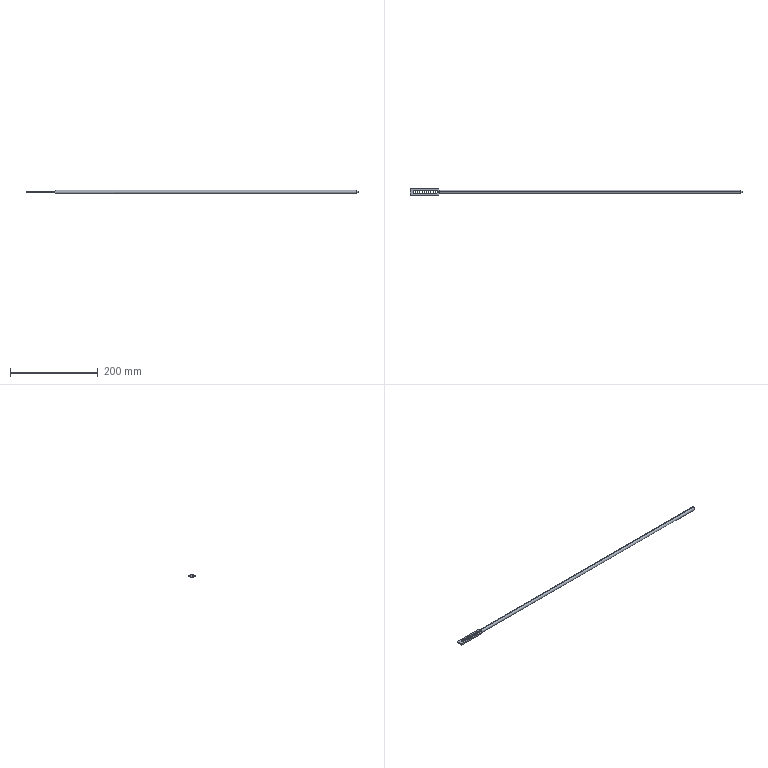Part | SolidWorks | 1 solid | 36 faces | box 757 x 14 x 8 mm | volume 36849 mm3 | cylinder 23 | plane 8 | cone 5 | commonest cylinder face diameters 6.1 x21 8 x2
STEP:
#1=CARTESIAN_POINT('',(67.,3.597,1.75));
#2=VERTEX_POINT('',#1);
#3=CARTESIAN_POINT('',(67.,0.,4.));
#4=VERTEX_POINT('',#3);
#5=CARTESIAN_POINT('',(67.,0.,0.));
#6=DIRECTION('',(1.,0.,0.));
#7=DIRECTION('',(0.,0.,-1.));
#8=AXIS2_PLACEMENT_3D('',#5,#6,#7);
#9=CIRCLE('',#8,4.);
#10=EDGE_CURVE('',#2,#4,#9,.T.);
#11=ORIENTED_EDGE('',*,*,#10,.T.);
#12=CARTESIAN_POINT('',(754.,0.,4.));
#13=VERTEX_POINT('',#12);
#14=CARTESIAN_POINT('',(757.,0.,4.));
#15=DIRECTION('',(1.,0.,0.));
#16=VECTOR('',#15,1000.);
#17=LINE('',#14,#16);
#18=EDGE_CURVE('',#4,#13,#17,.T.);
#19=ORIENTED_EDGE('',*,*,#18,.T.);
#20=CARTESIAN_POINT('',(754.,4.,0.));
#21=VERTEX_POINT('',#20);
#22=CARTESIAN_POINT('',(754.,0.,0.));
#23=DIRECTION('',(-1.,0.,0.));
#24=DIRECTION('',(0.,0.,-1.));
#25=AXIS2_PLACEMENT_3D('',#22,#23,#24);
#26=CIRCLE('',#25,4.);
#27=EDGE_CURVE('',#13,#21,#26,.T.);
#28=ORIENTED_EDGE('',*,*,#27,.T.);
#29=CARTESIAN_POINT('',(754.,0.,-4.));
#30=VERTEX_POINT('',#29);
#31=CARTESIAN_POINT('',(754.,0.,0.));
#32=DIRECTION('',(-1.,0.,0.));
#33=DIRECTION('',(0.,0.,-1.));
#34=AXIS2_PLACEMENT_3D('',#31,#32,#33);
#35=CIRCLE('',#34,4.);
#36=EDGE_CURVE('',#21,#30,#35,.T.);
#37=ORIENTED_EDGE('',*,*,#36,.T.);
#38=CARTESIAN_POINT('',(67.,0.,-4.));
#39=VERTEX_POINT('',#38);
#40=CARTESIAN_POINT('',(757.,0.,-4.));
#41=DIRECTION('',(1.,0.,0.));
#42=VECTOR('',#41,1000.);
#43=LINE('',#40,#42);
#44=EDGE_CURVE('',#39,#30,#43,.T.);
#45=ORIENTED_EDGE('',*,*,#44,.F.);
#46=CARTESIAN_POINT('',(67.,3.597,-1.75));
#47=VERTEX_POINT('',#46);
#48=CARTESIAN_POINT('',(67.,0.,0.));
#49=DIRECTION('',(1.,0.,0.));
#50=DIRECTION('',(0.,0.,-1.));
#51=AXIS2_PLACEMENT_3D('',#48,#49,#50);
#52=CIRCLE('',#51,4.);
#53=EDGE_CURVE('',#39,#47,#52,.T.);
#54=ORIENTED_EDGE('',*,*,#53,.T.);
#55=CARTESIAN_POINT('',(67.903,3.597,-1.75));
#56=VERTEX_POINT('',#55);
#57=CARTESIAN_POINT('',(68.,3.597,-1.75));
#58=DIRECTION('',(1.,0.,0.));
#59=VECTOR('',#58,1000.);
#60=LINE('',#57,#59);
#61=EDGE_CURVE('',#47,#56,#60,.T.);
#62=ORIENTED_EDGE('',*,*,#61,.T.);
#63=CARTESIAN_POINT('',(67.903,3.597,1.75));
#64=VERTEX_POINT('',#63);
#65=CARTESIAN_POINT('',(67.903,3.597,-1.75));
#66=CARTESIAN_POINT('',(67.356,4.144,-0.6253));
#67=CARTESIAN_POINT('',(67.356,4.144,0.6253));
#68=CARTESIAN_POINT('',(67.903,3.597,1.75));
#69=(BOUNDED_CURVE()B_SPLINE_CURVE(3,(#65,#66,#67,#68),.UNSPECIFIED.,.F.,.F.)B_SPLINE_CURVE_WITH_KNOTS((4,4),(2.689,3.594),.UNSPECIFIED.)CURVE()GEOMETRIC_REPRESENTATION_ITEM()RATIONAL_B_SPLINE_CURVE((1.,0.9328,0.9328,1.))REPRESENTATION_ITEM(''));
#70=EDGE_CURVE('',#56,#64,#69,.T.);
#71=ORIENTED_EDGE('',*,*,#70,.T.);
#72=CARTESIAN_POINT('',(0.,3.597,1.75));
#73=DIRECTION('',(-1.,0.,0.));
#74=VECTOR('',#73,1000.);
#75=LINE('',#72,#74);
#76=EDGE_CURVE('',#64,#2,#75,.T.);
#77=ORIENTED_EDGE('',*,*,#76,.T.);
#78=EDGE_LOOP('',(#11,#19,#28,#37,#45,#54,#62,#71,#77));
#79=FACE_OUTER_BOUND('',#78,.T.);
#80=CARTESIAN_POINT('',(757.,0.,0.));
#81=DIRECTION('',(1.,0.,0.));
#82=DIRECTION('',(0.,0.,-1.));
#83=AXIS2_PLACEMENT_3D('',#80,#81,#82);
#84=CYLINDRICAL_SURFACE('',#83,4.);
#85=ADVANCED_FACE('',(#79),#84,.T.);
#86=CARTESIAN_POINT('',(67.,-3.597,-1.75));
#87=VERTEX_POINT('',#86);
#88=CARTESIAN_POINT('',(65.678,0.,-1.75));
#89=VERTEX_POINT('',#88);
#90=CARTESIAN_POINT('',(67.,-3.597,-1.75));
#91=CARTESIAN_POINT('',(66.849,-3.312,-1.75));
#92=CARTESIAN_POINT('',(66.701,-3.025,-1.75));
#93=CARTESIAN_POINT('',(66.416,-2.448,-1.75));
#94=CARTESIAN_POINT('',(66.277,-2.157,-1.75));
#95=CARTESIAN_POINT('',(66.024,-1.564,-1.75));
#96=CARTESIAN_POINT('',(65.907,-1.262,-1.75));
#97=CARTESIAN_POINT('',(65.777,-0.7984,-1.75));
#98=CARTESIAN_POINT('',(65.741,-0.642,-1.75));
#99=CARTESIAN_POINT('',(65.692,-0.3236,-1.75));
#100=CARTESIAN_POINT('',(65.678,-0.1604,-1.75));
#101=CARTESIAN_POINT('',(65.678,0.,-1.75));
#102=B_SPLINE_CURVE_WITH_KNOTS('',3,(#90,#91,#92,#93,#94,#95,#96,#97,#98,#99,#100,#101),.UNSPECIFIED.,.F.,.F.,(4,2,2,2,2,4),(0.,0.0009664,0.001933,0.002899,0.003382,0.003866),.UNSPECIFIED.);
#103=EDGE_CURVE('',#87,#89,#102,.T.);
#104=ORIENTED_EDGE('',*,*,#103,.T.);
#105=CARTESIAN_POINT('',(67.,0.,-4.));
#106=DIRECTION('',(0.5065,0.,-0.8622));
#107=VECTOR('',#106,1000.);
#108=LINE('',#105,#107);
#109=EDGE_CURVE('',#89,#39,#108,.T.);
#110=ORIENTED_EDGE('',*,*,#109,.T.);
#111=CARTESIAN_POINT('',(67.,0.,0.));
#112=DIRECTION('',(1.,0.,0.));
#113=DIRECTION('',(0.,0.,-1.));
#114=AXIS2_PLACEMENT_3D('',#111,#112,#113);
#115=CIRCLE('',#114,4.);
#116=EDGE_CURVE('',#87,#39,#115,.T.);
#117=ORIENTED_EDGE('',*,*,#116,.F.);
#118=EDGE_LOOP('',(#104,#110,#117));
#119=FACE_OUTER_BOUND('',#118,.T.);
#120=CARTESIAN_POINT('',(67.,0.,0.));
#121=DIRECTION('',(1.,0.,0.));
#122=DIRECTION('',(0.,0.,-1.));
#123=AXIS2_PLACEMENT_3D('',#120,#121,#122);
#124=CONICAL_SURFACE('',#123,4.,1.04);
#125=ADVANCED_FACE('',(#119),#124,.T.);
#126=CARTESIAN_POINT('',(757.,-1.5,0.));
#127=VERTEX_POINT('',#126);
#128=CARTESIAN_POINT('',(757.,1.5,0.));
#129=VERTEX_POINT('',#128);
#130=CARTESIAN_POINT('',(757.,0.,0.));
#131=DIRECTION('',(-1.,0.,0.));
#132=DIRECTION('',(0.,-1.,0.));
#133=AXIS2_PLACEMENT_3D('',#130,#131,#132);
#134=CIRCLE('',#133,1.5);
#135=EDGE_CURVE('',#127,#129,#134,.T.);
#136=ORIENTED_EDGE('',*,*,#135,.T.);
#137=CARTESIAN_POINT('',(754.,4.,0.));
#138=DIRECTION('',(-0.7682,0.6402,0.));
#139=VECTOR('',#138,1000.);
#140=LINE('',#137,#139);
#141=EDGE_CURVE('',#129,#21,#140,.T.);
#142=ORIENTED_EDGE('',*,*,#141,.T.);
#143=ORIENTED_EDGE('',*,*,#27,.F.);
#144=CARTESIAN_POINT('',(754.,-4.,0.));
#145=VERTEX_POINT('',#144);
#146=CARTESIAN_POINT('',(754.,0.,0.));
#147=DIRECTION('',(-1.,0.,0.));
#148=DIRECTION('',(0.,0.,-1.));
#149=AXIS2_PLACEMENT_3D('',#146,#147,#148);
#150=CIRCLE('',#149,4.);
#151=EDGE_CURVE('',#145,#13,#150,.T.);
#152=ORIENTED_EDGE('',*,*,#151,.F.);
#153=CARTESIAN_POINT('',(754.,-4.,0.));
#154=DIRECTION('',(-0.7682,-0.6402,0.));
#155=VECTOR('',#154,1000.);
#156=LINE('',#153,#155);
#157=EDGE_CURVE('',#127,#145,#156,.T.);
#158=ORIENTED_EDGE('',*,*,#157,.F.);
#159=EDGE_LOOP('',(#136,#142,#143,#152,#158));
#160=FACE_OUTER_BOUND('',#159,.T.);
#161=CARTESIAN_POINT('',(754.,0.,0.));
#162=DIRECTION('',(-1.,0.,0.));
#163=DIRECTION('',(0.,-1.,0.));
#164=AXIS2_PLACEMENT_3D('',#161,#162,#163);
#165=CONICAL_SURFACE('',#164,4.,0.6947);
#166=ADVANCED_FACE('',(#160),#165,.T.);
#167=CARTESIAN_POINT('',(12.5,1.747,1.75));
#168=VERTEX_POINT('',#167);
#169=CARTESIAN_POINT('',(6.95,0.,1.75));
#170=VERTEX_POINT('',#169);
#171=CARTESIAN_POINT('',(10.,0.,1.75));
#172=DIRECTION('',(0.,0.,1.));
#173=DIRECTION('',(-1.,0.,0.));
#174=AXIS2_PLACEMENT_3D('',#171,#172,#173);
#175=CIRCLE('',#174,3.05);
#176=EDGE_CURVE('',#168,#170,#175,.T.);
#177=ORIENTED_EDGE('',*,*,#176,.T.);
#178=CARTESIAN_POINT('',(6.95,0.,-1.75));
#179=VERTEX_POINT('',#178);
#180=CARTESIAN_POINT('',(6.95,0.,7.));
#181=DIRECTION('',(0.,0.,-1.));
#182=VECTOR('',#181,1000.);
#183=LINE('',#180,#182);
#184=EDGE_CURVE('',#170,#179,#183,.T.);
#185=ORIENTED_EDGE('',*,*,#184,.T.);
#186=CARTESIAN_POINT('',(12.5,1.747,-1.75));
#187=VERTEX_POINT('',#186);
#188=CARTESIAN_POINT('',(10.,0.,-1.75));
#189=DIRECTION('',(0.,0.,-1.));
#190=DIRECTION('',(-1.,0.,0.));
#191=AXIS2_PLACEMENT_3D('',#188,#189,#190);
#192=CIRCLE('',#191,3.05);
#193=EDGE_CURVE('',#179,#187,#192,.T.);
#194=ORIENTED_EDGE('',*,*,#193,.T.);
#195=CARTESIAN_POINT('',(12.5,1.747,7.));
#196=DIRECTION('',(0.,0.,1.));
#197=VECTOR('',#196,1000.);
#198=LINE('',#195,#197);
#199=EDGE_CURVE('',#187,#168,#198,.T.);
#200=ORIENTED_EDGE('',*,*,#199,.T.);
#201=EDGE_LOOP('',(#177,#185,#194,#200));
#202=FACE_OUTER_BOUND('',#201,.T.);
#203=CARTESIAN_POINT('',(10.,0.,7.));
#204=DIRECTION('',(0.,0.,-1.));
#205=DIRECTION('',(-1.,0.,0.));
#206=AXIS2_PLACEMENT_3D('',#203,#204,#205);
#207=CYLINDRICAL_SURFACE('',#206,3.05);
#208=ADVANCED_FACE('',(#202),#207,.F.);
#209=ORIENTED_EDGE('',*,*,#18,.F.);
#210=CARTESIAN_POINT('',(67.,-3.597,1.75));
#211=VERTEX_POINT('',#210);
#212=CARTESIAN_POINT('',(67.,0.,0.));
#213=DIRECTION('',(1.,0.,0.));
#214=DIRECTION('',(0.,0.,-1.));
#215=AXIS2_PLACEMENT_3D('',#212,#213,#214);
#216=CIRCLE('',#215,4.);
#217=EDGE_CURVE('',#4,#211,#216,.T.);
#218=ORIENTED_EDGE('',*,*,#217,.T.);
#219=CARTESIAN_POINT('',(67.903,-3.597,1.75));
#220=VERTEX_POINT('',#219);
#221=CARTESIAN_POINT('',(0.,-3.597,1.75));
#222=DIRECTION('',(1.,0.,0.));
#223=VECTOR('',#222,1000.);
#224=LINE('',#221,#223);
#225=EDGE_CURVE('',#211,#220,#224,.T.);
#226=ORIENTED_EDGE('',*,*,#225,.T.);
#227=CARTESIAN_POINT('',(67.903,-3.597,-1.75));
#228=VERTEX_POINT('',#227);
#229=CARTESIAN_POINT('',(67.903,-3.597,1.75));
#230=CARTESIAN_POINT('',(67.356,-4.144,0.6253));
#231=CARTESIAN_POINT('',(67.356,-4.144,-0.6253));
#232=CARTESIAN_POINT('',(67.903,-3.597,-1.75));
#233=(BOUNDED_CURVE()B_SPLINE_CURVE(3,(#229,#230,#231,#232),.UNSPECIFIED.,.F.,.T.)B_SPLINE_CURVE_WITH_KNOTS((4,4),(2.689,3.594),.UNSPECIFIED.)CURVE()GEOMETRIC_REPRESENTATION_ITEM()RATIONAL_B_SPLINE_CURVE((1.,0.9328,0.9328,1.))REPRESENTATION_ITEM(''));
#234=EDGE_CURVE('',#220,#228,#233,.T.);
#235=ORIENTED_EDGE('',*,*,#234,.T.);
#236=CARTESIAN_POINT('',(68.,-3.597,-1.75));
#237=DIRECTION('',(-1.,0.,0.));
#238=VECTOR('',#237,1000.);
#239=LINE('',#236,#238);
#240=EDGE_CURVE('',#228,#87,#239,.T.);
#241=ORIENTED_EDGE('',*,*,#240,.T.);
#242=ORIENTED_EDGE('',*,*,#116,.T.);
#243=ORIENTED_EDGE('',*,*,#44,.T.);
#244=CARTESIAN_POINT('',(754.,0.,0.));
#245=DIRECTION('',(-1.,0.,0.));
#246=DIRECTION('',(0.,0.,-1.));
#247=AXIS2_PLACEMENT_3D('',#244,#245,#246);
#248=CIRCLE('',#247,4.);
#249=EDGE_CURVE('',#30,#145,#248,.T.);
#250=ORIENTED_EDGE('',*,*,#249,.T.);
#251=ORIENTED_EDGE('',*,*,#151,.T.);
#252=EDGE_LOOP('',(#209,#218,#226,#235,#241,#242,#243,#250,#251));
#253=FACE_OUTER_BOUND('',#252,.T.);
#254=CARTESIAN_POINT('',(757.,0.,0.));
#255=DIRECTION('',(1.,0.,0.));
#256=DIRECTION('',(0.,0.,-1.));
#257=AXIS2_PLACEMENT_3D('',#254,#255,#256);
#258=CYLINDRICAL_SURFACE('',#257,4.);
#259=ADVANCED_FACE('',(#253),#258,.T.);
#260=ORIENTED_EDGE('',*,*,#234,.F.);
#261=CARTESIAN_POINT('',(64.5,-7.,1.75));
#262=VERTEX_POINT('',#261);
#263=CARTESIAN_POINT('',(68.,-3.5,1.75));
#264=DIRECTION('',(0.7071,0.7071,0.));
#265=VECTOR('',#264,1000.);
#266=LINE('',#263,#265);
#267=EDGE_CURVE('',#262,#220,#266,.T.);
#268=ORIENTED_EDGE('',*,*,#267,.F.);
#269=CARTESIAN_POINT('',(64.5,-7.,-1.75));
#270=VERTEX_POINT('',#269);
#271=CARTESIAN_POINT('',(64.5,-7.,1.75));
#272=DIRECTION('',(0.,0.,1.));
#273=VECTOR('',#272,1000.);
#274=LINE('',#271,#273);
#275=EDGE_CURVE('',#270,#262,#274,.T.);
#276=ORIENTED_EDGE('',*,*,#275,.F.);
#277=CARTESIAN_POINT('',(68.,-3.5,-1.75));
#278=DIRECTION('',(-0.7071,-0.7071,0.));
#279=VECTOR('',#278,1000.);
#280=LINE('',#277,#279);
#281=EDGE_CURVE('',#228,#270,#280,.T.);
#282=ORIENTED_EDGE('',*,*,#281,.F.);
#283=EDGE_LOOP('',(#260,#268,#276,#282));
#284=FACE_OUTER_BOUND('',#283,.T.);
#285=CARTESIAN_POINT('',(68.,-3.5,1.75));
#286=DIRECTION('',(-0.7071,0.7071,0.));
#287=DIRECTION('',(-0.7071,-0.7071,0.));
#288=AXIS2_PLACEMENT_3D('',#285,#286,#287);
#289=PLANE('',#288);
#290=ADVANCED_FACE('',(#284),#289,.F.);
#291=ORIENTED_EDGE('',*,*,#10,.F.);
#292=CARTESIAN_POINT('',(67.,3.597,1.75));
#293=CARTESIAN_POINT('',(66.849,3.311,1.75));
#294=CARTESIAN_POINT('',(66.701,3.024,1.75));
#295=CARTESIAN_POINT('',(66.414,2.445,1.75));
#296=CARTESIAN_POINT('',(66.276,2.153,1.75));
#297=CARTESIAN_POINT('',(66.022,1.559,1.75));
#298=CARTESIAN_POINT('',(65.905,1.255,1.75));
#299=CARTESIAN_POINT('',(65.775,0.7905,1.75));
#300=CARTESIAN_POINT('',(65.74,0.6336,1.75));
#301=CARTESIAN_POINT('',(65.691,0.3142,1.75));
#302=CARTESIAN_POINT('',(65.678,0.1505,1.75));
#303=CARTESIAN_POINT('',(65.679,-0.3318,1.75));
#304=CARTESIAN_POINT('',(65.734,-0.6464,1.75));
#305=CARTESIAN_POINT('',(65.909,-1.267,1.75));
#306=CARTESIAN_POINT('',(66.026,-1.569,1.75));
#307=CARTESIAN_POINT('',(66.279,-2.16,1.75));
#308=CARTESIAN_POINT('',(66.417,-2.45,1.75));
#309=CARTESIAN_POINT('',(66.702,-3.027,1.75));
#310=CARTESIAN_POINT('',(66.85,-3.312,1.75));
#311=CARTESIAN_POINT('',(67.,-3.597,1.75));
#312=B_SPLINE_CURVE_WITH_KNOTS('',3,(#292,#293,#294,#295,#296,#297,#298,#299,#300,#301,#302,#303,#304,#305,#306,#307,#308,#309,#310,#311),.UNSPECIFIED.,.F.,.F.,(4,2,2,2,2,2,2,2,2,4),(0.,0.000969,0.001938,0.002907,0.003392,0.003876,0.004845,0.005814,0.006783,0.007752),.UNSPECIFIED.);
#313=EDGE_CURVE('',#2,#211,#312,.T.);
#314=ORIENTED_EDGE('',*,*,#313,.T.);
#315=ORIENTED_EDGE('',*,*,#217,.F.);
#316=EDGE_LOOP('',(#291,#314,#315));
#317=FACE_OUTER_BOUND('',#316,.T.);
#318=CARTESIAN_POINT('',(67.,0.,0.));
#319=DIRECTION('',(1.,0.,0.));
#320=DIRECTION('',(0.,0.,-1.));
#321=AXIS2_PLACEMENT_3D('',#318,#319,#320);
#322=CONICAL_SURFACE('',#321,4.,1.04);
#323=ADVANCED_FACE('',(#317),#322,.T.);
#324=CARTESIAN_POINT('',(64.5,7.,-1.75));
#325=VERTEX_POINT('',#324);
#326=CARTESIAN_POINT('',(64.5,7.,-1.75));
#327=DIRECTION('',(-0.7071,0.7071,0.));
#328=VECTOR('',#327,1000.);
#329=LINE('',#326,#328);
#330=EDGE_CURVE('',#56,#325,#329,.T.);
#331=ORIENTED_EDGE('',*,*,#330,.T.);
#332=CARTESIAN_POINT('',(64.5,7.,1.75));
#333=VERTEX_POINT('',#332);
#334=CARTESIAN_POINT('',(64.5,7.,0.));
#335=DIRECTION('',(0.,0.,1.));
#336=VECTOR('',#335,1000.);
#337=LINE('',#334,#336);
#338=EDGE_CURVE('',#325,#333,#337,.T.);
#339=ORIENTED_EDGE('',*,*,#338,.T.);
#340=CARTESIAN_POINT('',(64.5,7.,1.75));
#341=DIRECTION('',(0.7071,-0.7071,0.));
#342=VECTOR('',#341,1000.);
#343=LINE('',#340,#342);
#344=EDGE_CURVE('',#333,#64,#343,.T.);
#345=ORIENTED_EDGE('',*,*,#344,.T.);
#346=ORIENTED_EDGE('',*,*,#70,.F.);
#347=EDGE_LOOP('',(#331,#339,#345,#346));
#348=FACE_OUTER_BOUND('',#347,.T.);
#349=CARTESIAN_POINT('',(64.5,7.,0.));
#350=DIRECTION('',(0.7071,0.7071,0.));
#351=DIRECTION('',(-0.7071,0.7071,0.));
#352=AXIS2_PLACEMENT_3D('',#349,#350,#351);
#353=PLANE('',#352);
#354=ADVANCED_FACE('',(#348),#353,.T.);
#355=ORIENTED_EDGE('',*,*,#109,.F.);
#356=CARTESIAN_POINT('',(65.678,0.,-1.75));
#357=CARTESIAN_POINT('',(65.678,0.3225,-1.75));
#358=CARTESIAN_POINT('',(65.732,0.6381,-1.75));
#359=CARTESIAN_POINT('',(65.907,1.261,-1.75));
#360=CARTESIAN_POINT('',(66.024,1.564,-1.75));
#361=CARTESIAN_POINT('',(66.277,2.156,-1.75));
#362=CARTESIAN_POINT('',(66.415,2.447,-1.75));
#363=CARTESIAN_POINT('',(66.701,3.025,-1.75));
#364=CARTESIAN_POINT('',(66.849,3.312,-1.75));
#365=CARTESIAN_POINT('',(67.,3.597,-1.75));
#366=B_SPLINE_CURVE_WITH_KNOTS('',3,(#356,#357,#358,#359,#360,#361,#362,#363,#364,#365),.UNSPECIFIED.,.F.,.F.,(4,2,2,2,4),(0.003866,0.004837,0.005809,0.00678,0.007752),.UNSPECIFIED.);
#367=EDGE_CURVE('',#89,#47,#366,.T.);
#368=ORIENTED_EDGE('',*,*,#367,.T.);
#369=ORIENTED_EDGE('',*,*,#53,.F.);
#370=EDGE_LOOP('',(#355,#368,#369));
#371=FACE_OUTER_BOUND('',#370,.T.);
#372=CARTESIAN_POINT('',(67.,0.,0.));
#373=DIRECTION('',(1.,0.,0.));
#374=DIRECTION('',(0.,0.,-1.));
#375=AXIS2_PLACEMENT_3D('',#372,#373,#374);
#376=CONICAL_SURFACE('',#375,4.,1.04);
#377=ADVANCED_FACE('',(#371),#376,.T.);
#378=ORIENTED_EDGE('',*,*,#141,.F.);
#379=CARTESIAN_POINT('',(757.,0.,0.));
#380=DIRECTION('',(-1.,0.,0.));
#381=DIRECTION('',(0.,-1.,0.));
#382=AXIS2_PLACEMENT_3D('',#379,#380,#381);
#383=CIRCLE('',#382,1.5);
#384=EDGE_CURVE('',#129,#127,#383,.T.);
#385=ORIENTED_EDGE('',*,*,#384,.T.);
#386=ORIENTED_EDGE('',*,*,#157,.T.);
#387=ORIENTED_EDGE('',*,*,#249,.F.);
#388=ORIENTED_EDGE('',*,*,#36,.F.);
#389=EDGE_LOOP('',(#378,#385,#386,#387,#388));
#390=FACE_OUTER_BOUND('',#389,.T.);
#391=CARTESIAN_POINT('',(754.,0.,0.));
#392=DIRECTION('',(-1.,0.,0.));
#393=DIRECTION('',(0.,-1.,0.));
#394=AXIS2_PLACEMENT_3D('',#391,#392,#393);
#395=CONICAL_SURFACE('',#394,4.,0.6947);
#396=ADVANCED_FACE('',(#390),#395,.T.);
#397=ORIENTED_EDGE('',*,*,#281,.T.);
#398=CARTESIAN_POINT('',(0.,-7.,-1.75));
#399=VERTEX_POINT('',#398);
#400=CARTESIAN_POINT('',(68.,-7.,-1.75));
#401=DIRECTION('',(1.,0.,0.));
#402=VECTOR('',#401,1000.);
#403=LINE('',#400,#402);
#404=EDGE_CURVE('',#399,#270,#403,.T.);
#405=ORIENTED_EDGE('',*,*,#404,.F.);
#406=CARTESIAN_POINT('',(0.,7.,-1.75));
#407=VERTEX_POINT('',#406);
#408=CARTESIAN_POINT('',(0.,7.,-1.75));
#409=DIRECTION('',(0.,-1.,0.));
#410=VECTOR('',#409,1000.);
#411=LINE('',#408,#410);
#412=EDGE_CURVE('',#407,#399,#411,.T.);
#413=ORIENTED_EDGE('',*,*,#412,.F.);
#414=CARTESIAN_POINT('',(68.,7.,-1.75));
#415=DIRECTION('',(-1.,0.,0.));
#416=VECTOR('',#415,1000.);
#417=LINE('',#414,#416);
#418=EDGE_CURVE('',#325,#407,#417,.T.);
#419=ORIENTED_EDGE('',*,*,#418,.F.);
#420=ORIENTED_EDGE('',*,*,#330,.F.);
#421=ORIENTED_EDGE('',*,*,#61,.F.);
#422=ORIENTED_EDGE('',*,*,#367,.F.);
#423=ORIENTED_EDGE('',*,*,#103,.F.);
#424=ORIENTED_EDGE('',*,*,#240,.F.);
#425=EDGE_LOOP('',(#397,#405,#413,#419,#420,#421,#422,#423,#424));
#426=FACE_OUTER_BOUND('',#425,.T.);
#427=CARTESIAN_POINT('',(22.5,-1.747,-1.75));
#428=VERTEX_POINT('',#427);
#429=CARTESIAN_POINT('',(17.5,-1.747,-1.75));
#430=VERTEX_POINT('',#429);
#431=CARTESIAN_POINT('',(20.,0.,-1.75));
#432=DIRECTION('',(0.,0.,-1.));
#433=DIRECTION('',(-1.,0.,0.));
#434=AXIS2_PLACEMENT_3D('',#431,#432,#433);
#435=CIRCLE('',#434,3.05);
#436=EDGE_CURVE('',#428,#430,#435,.T.);
#437=ORIENTED_EDGE('',*,*,#436,.F.);
#438=CARTESIAN_POINT('',(27.5,-1.747,-1.75));
#439=VERTEX_POINT('',#438);
#440=CARTESIAN_POINT('',(25.,0.,-1.75));
#441=DIRECTION('',(0.,0.,-1.));
#442=DIRECTION('',(-1.,0.,0.));
#443=AXIS2_PLACEMENT_3D('',#440,#441,#442);
#444=CIRCLE('',#443,3.05);
#445=EDGE_CURVE('',#439,#428,#444,.T.);
#446=ORIENTED_EDGE('',*,*,#445,.F.);
#447=CARTESIAN_POINT('',(32.5,-1.747,-1.75));
#448=VERTEX_POINT('',#447);
#449=CARTESIAN_POINT('',(30.,0.,-1.75));
#450=DIRECTION('',(0.,0.,-1.));
#451=DIRECTION('',(-1.,0.,0.));
#452=AXIS2_PLACEMENT_3D('',#449,#450,#451);
#453=CIRCLE('',#452,3.05);
#454=EDGE_CURVE('',#448,#439,#453,.T.);
#455=ORIENTED_EDGE('',*,*,#454,.F.);
#456=CARTESIAN_POINT('',(37.5,-1.747,-1.75));
#457=VERTEX_POINT('',#456);
#458=CARTESIAN_POINT('',(35.,0.,-1.75));
#459=DIRECTION('',(0.,0.,-1.));
#460=DIRECTION('',(-1.,0.,0.));
#461=AXIS2_PLACEMENT_3D('',#458,#459,#460);
#462=CIRCLE('',#461,3.05);
#463=EDGE_CURVE('',#457,#448,#462,.T.);
#464=ORIENTED_EDGE('',*,*,#463,.F.);
#465=CARTESIAN_POINT('',(42.5,-1.747,-1.75));
#466=VERTEX_POINT('',#465);
#467=CARTESIAN_POINT('',(40.,0.,-1.75));
#468=DIRECTION('',(0.,0.,-1.));
#469=DIRECTION('',(-1.,0.,0.));
#470=AXIS2_PLACEMENT_3D('',#467,#468,#469);
#471=CIRCLE('',#470,3.05);
#472=EDGE_CURVE('',#466,#457,#471,.T.);
#473=ORIENTED_EDGE('',*,*,#472,.F.);
#474=CARTESIAN_POINT('',(47.5,-1.747,-1.75));
#475=VERTEX_POINT('',#474);
#476=CARTESIAN_POINT('',(45.,0.,-1.75));
#477=DIRECTION('',(0.,0.,-1.));
#478=DIRECTION('',(-1.,0.,0.));
#479=AXIS2_PLACEMENT_3D('',#476,#477,#478);
#480=CIRCLE('',#479,3.05);
#481=EDGE_CURVE('',#475,#466,#480,.T.);
#482=ORIENTED_EDGE('',*,*,#481,.F.);
#483=CARTESIAN_POINT('',(52.5,-1.747,-1.75));
#484=VERTEX_POINT('',#483);
#485=CARTESIAN_POINT('',(50.,0.,-1.75));
#486=DIRECTION('',(0.,0.,-1.));
#487=DIRECTION('',(-1.,0.,0.));
#488=AXIS2_PLACEMENT_3D('',#485,#486,#487);
#489=CIRCLE('',#488,3.05);
#490=EDGE_CURVE('',#484,#475,#489,.T.);
#491=ORIENTED_EDGE('',*,*,#490,.F.);
#492=CARTESIAN_POINT('',(57.5,-1.747,-1.75));
#493=VERTEX_POINT('',#492);
#494=CARTESIAN_POINT('',(55.,0.,-1.75));
#495=DIRECTION('',(0.,0.,-1.));
#496=DIRECTION('',(-1.,0.,0.));
#497=AXIS2_PLACEMENT_3D('',#494,#495,#496);
#498=CIRCLE('',#497,3.05);
#499=EDGE_CURVE('',#493,#484,#498,.T.);
#500=ORIENTED_EDGE('',*,*,#499,.F.);
#501=CARTESIAN_POINT('',(57.5,1.747,-1.75));
#502=VERTEX_POINT('',#501);
#503=CARTESIAN_POINT('',(60.,0.,-1.75));
#504=DIRECTION('',(0.,0.,-1.));
#505=DIRECTION('',(-1.,0.,0.));
#506=AXIS2_PLACEMENT_3D('',#503,#504,#505);
#507=CIRCLE('',#506,3.05);
#508=EDGE_CURVE('',#502,#493,#507,.T.);
#509=ORIENTED_EDGE('',*,*,#508,.F.);
#510=CARTESIAN_POINT('',(52.5,1.747,-1.75));
#511=VERTEX_POINT('',#510);
#512=CARTESIAN_POINT('',(55.,0.,-1.75));
#513=DIRECTION('',(0.,0.,-1.));
#514=DIRECTION('',(-1.,0.,0.));
#515=AXIS2_PLACEMENT_3D('',#512,#513,#514);
#516=CIRCLE('',#515,3.05);
#517=EDGE_CURVE('',#511,#502,#516,.T.);
#518=ORIENTED_EDGE('',*,*,#517,.F.);
#519=CARTESIAN_POINT('',(47.5,1.747,-1.75));
#520=VERTEX_POINT('',#519);
#521=CARTESIAN_POINT('',(50.,0.,-1.75));
#522=DIRECTION('',(0.,0.,-1.));
#523=DIRECTION('',(-1.,0.,0.));
#524=AXIS2_PLACEMENT_3D('',#521,#522,#523);
#525=CIRCLE('',#524,3.05);
#526=EDGE_CURVE('',#520,#511,#525,.T.);
#527=ORIENTED_EDGE('',*,*,#526,.F.);
#528=CARTESIAN_POINT('',(42.5,1.747,-1.75));
#529=VERTEX_POINT('',#528);
#530=CARTESIAN_POINT('',(45.,0.,-1.75));
#531=DIRECTION('',(0.,0.,-1.));
#532=DIRECTION('',(-1.,0.,0.));
#533=AXIS2_PLACEMENT_3D('',#530,#531,#532);
#534=CIRCLE('',#533,3.05);
#535=EDGE_CURVE('',#529,#520,#534,.T.);
#536=ORIENTED_EDGE('',*,*,#535,.F.);
#537=CARTESIAN_POINT('',(37.5,1.747,-1.75));
#538=VERTEX_POINT('',#537);
#539=CARTESIAN_POINT('',(40.,0.,-1.75));
#540=DIRECTION('',(0.,0.,-1.));
#541=DIRECTION('',(-1.,0.,0.));
#542=AXIS2_PLACEMENT_3D('',#539,#540,#541);
#543=CIRCLE('',#542,3.05);
#544=EDGE_CURVE('',#538,#529,#543,.T.);
#545=ORIENTED_EDGE('',*,*,#544,.F.);
#546=CARTESIAN_POINT('',(32.5,1.747,-1.75));
#547=VERTEX_POINT('',#546);
#548=CARTESIAN_POINT('',(35.,0.,-1.75));
#549=DIRECTION('',(0.,0.,-1.));
#550=DIRECTION('',(-1.,0.,0.));
#551=AXIS2_PLACEMENT_3D('',#548,#549,#550);
#552=CIRCLE('',#551,3.05);
#553=EDGE_CURVE('',#547,#538,#552,.T.);
#554=ORIENTED_EDGE('',*,*,#553,.F.);
#555=CARTESIAN_POINT('',(27.5,1.747,-1.75));
#556=VERTEX_POINT('',#555);
#557=CARTESIAN_POINT('',(30.,0.,-1.75));
#558=DIRECTION('',(0.,0.,-1.));
#559=DIRECTION('',(-1.,0.,0.));
#560=AXIS2_PLACEMENT_3D('',#557,#558,#559);
#561=CIRCLE('',#560,3.05);
#562=EDGE_CURVE('',#556,#547,#561,.T.);
#563=ORIENTED_EDGE('',*,*,#562,.F.);
#564=CARTESIAN_POINT('',(22.5,1.747,-1.75));
#565=VERTEX_POINT('',#564);
#566=CARTESIAN_POINT('',(25.,0.,-1.75));
#567=DIRECTION('',(0.,0.,-1.));
#568=DIRECTION('',(-1.,0.,0.));
#569=AXIS2_PLACEMENT_3D('',#566,#567,#568);
#570=CIRCLE('',#569,3.05);
#571=EDGE_CURVE('',#565,#556,#570,.T.);
#572=ORIENTED_EDGE('',*,*,#571,.F.);
#573=CARTESIAN_POINT('',(17.5,1.747,-1.75));
#574=VERTEX_POINT('',#573);
#575=CARTESIAN_POINT('',(20.,0.,-1.75));
#576=DIRECTION('',(0.,0.,-1.));
#577=DIRECTION('',(-1.,0.,0.));
#578=AXIS2_PLACEMENT_3D('',#575,#576,#577);
#579=CIRCLE('',#578,3.05);
#580=EDGE_CURVE('',#574,#565,#579,.T.);
#581=ORIENTED_EDGE('',*,*,#580,.F.);
#582=CARTESIAN_POINT('',(15.,0.,-1.75));
#583=DIRECTION('',(0.,0.,-1.));
#584=DIRECTION('',(-1.,0.,0.));
#585=AXIS2_PLACEMENT_3D('',#582,#583,#584);
#586=CIRCLE('',#585,3.05);
#587=EDGE_CURVE('',#187,#574,#586,.T.);
#588=ORIENTED_EDGE('',*,*,#587,.F.);
#589=ORIENTED_EDGE('',*,*,#193,.F.);
#590=CARTESIAN_POINT('',(12.5,-1.747,-1.75));
#591=VERTEX_POINT('',#590);
#592=CARTESIAN_POINT('',(10.,0.,-1.75));
#593=DIRECTION('',(0.,0.,-1.));
#594=DIRECTION('',(-1.,0.,0.));
#595=AXIS2_PLACEMENT_3D('',#592,#593,#594);
#596=CIRCLE('',#595,3.05);
#597=EDGE_CURVE('',#591,#179,#596,.T.);
#598=ORIENTED_EDGE('',*,*,#597,.F.);
#599=CARTESIAN_POINT('',(15.,0.,-1.75));
#600=DIRECTION('',(0.,0.,-1.));
#601=DIRECTION('',(-1.,0.,0.));
#602=AXIS2_PLACEMENT_3D('',#599,#600,#601);
#603=CIRCLE('',#602,3.05);
#604=EDGE_CURVE('',#430,#591,#603,.T.);
#605=ORIENTED_EDGE('',*,*,#604,.F.);
#606=EDGE_LOOP('',(#437,#446,#455,#464,#473,#482,#491,#500,#509,#518,#527,#536,#545,#554,#563,#572,#581,#588,#589,#598,#605));
#607=FACE_BOUND('',#606,.T.);
#608=CARTESIAN_POINT('',(68.,7.,-1.75));
#609=DIRECTION('',(0.,0.,1.));
#610=DIRECTION('',(1.,0.,0.));
#611=AXIS2_PLACEMENT_3D('',#608,#609,#610);
#612=PLANE('',#611);
#613=ADVANCED_FACE('',(#426,#607),#612,.F.);
#614=ORIENTED_EDGE('',*,*,#344,.F.);
#615=CARTESIAN_POINT('',(0.,7.,1.75));
#616=VERTEX_POINT('',#615);
#617=CARTESIAN_POINT('',(0.,7.,1.75));
#618=DIRECTION('',(1.,0.,0.));
#619=VECTOR('',#618,1000.);
#620=LINE('',#617,#619);
#621=EDGE_CURVE('',#616,#333,#620,.T.);
#622=ORIENTED_EDGE('',*,*,#621,.F.);
#623=CARTESIAN_POINT('',(0.,-7.,1.75));
#624=VERTEX_POINT('',#623);
#625=CARTESIAN_POINT('',(0.,7.,1.75));
#626=DIRECTION('',(0.,1.,0.));
#627=VECTOR('',#626,1000.);
#628=LINE('',#625,#627);
#629=EDGE_CURVE('',#624,#616,#628,.T.);
#630=ORIENTED_EDGE('',*,*,#629,.F.);
#631=CARTESIAN_POINT('',(0.,-7.,1.75));
#632=DIRECTION('',(-1.,0.,0.));
#633=VECTOR('',#632,1000.);
#634=LINE('',#631,#633);
#635=EDGE_CURVE('',#262,#624,#634,.T.);
#636=ORIENTED_EDGE('',*,*,#635,.F.);
#637=ORIENTED_EDGE('',*,*,#267,.T.);
#638=ORIENTED_EDGE('',*,*,#225,.F.);
#639=ORIENTED_EDGE('',*,*,#313,.F.);
#640=ORIENTED_EDGE('',*,*,#76,.F.);
#641=EDGE_LOOP('',(#614,#622,#630,#636,#637,#638,#639,#640));
#642=FACE_OUTER_BOUND('',#641,.T.);
#643=CARTESIAN_POINT('',(22.5,1.747,1.75));
#644=VERTEX_POINT('',#643);
#645=CARTESIAN_POINT('',(17.5,1.747,1.75));
#646=VERTEX_POINT('',#645);
#647=CARTESIAN_POINT('',(20.,0.,1.75));
#648=DIRECTION('',(0.,0.,1.));
#649=DIRECTION('',(-1.,0.,0.));
#650=AXIS2_PLACEMENT_3D('',#647,#648,#649);
#651=CIRCLE('',#650,3.05);
#652=EDGE_CURVE('',#644,#646,#651,.T.);
#653=ORIENTED_EDGE('',*,*,#652,.F.);
#654=CARTESIAN_POINT('',(27.5,1.747,1.75));
#655=VERTEX_POINT('',#654);
#656=CARTESIAN_POINT('',(25.,0.,1.75));
#657=DIRECTION('',(0.,0.,1.));
#658=DIRECTION('',(-1.,0.,0.));
#659=AXIS2_PLACEMENT_3D('',#656,#657,#658);
#660=CIRCLE('',#659,3.05);
#661=EDGE_CURVE('',#655,#644,#660,.T.);
#662=ORIENTED_EDGE('',*,*,#661,.F.);
#663=CARTESIAN_POINT('',(32.5,1.747,1.75));
#664=VERTEX_POINT('',#663);
#665=CARTESIAN_POINT('',(30.,0.,1.75));
#666=DIRECTION('',(0.,0.,1.));
#667=DIRECTION('',(-1.,0.,0.));
#668=AXIS2_PLACEMENT_3D('',#665,#666,#667);
#669=CIRCLE('',#668,3.05);
#670=EDGE_CURVE('',#664,#655,#669,.T.);
#671=ORIENTED_EDGE('',*,*,#670,.F.);
#672=CARTESIAN_POINT('',(37.5,1.747,1.75));
#673=VERTEX_POINT('',#672);
#674=CARTESIAN_POINT('',(35.,0.,1.75));
#675=DIRECTION('',(0.,0.,1.));
#676=DIRECTION('',(-1.,0.,0.));
#677=AXIS2_PLACEMENT_3D('',#674,#675,#676);
#678=CIRCLE('',#677,3.05);
#679=EDGE_CURVE('',#673,#664,#678,.T.);
#680=ORIENTED_EDGE('',*,*,#679,.F.);
#681=CARTESIAN_POINT('',(42.5,1.747,1.75));
#682=VERTEX_POINT('',#681);
#683=CARTESIAN_POINT('',(40.,0.,1.75));
#684=DIRECTION('',(0.,0.,1.));
#685=DIRECTION('',(-1.,0.,0.));
#686=AXIS2_PLACEMENT_3D('',#683,#684,#685);
#687=CIRCLE('',#686,3.05);
#688=EDGE_CURVE('',#682,#673,#687,.T.);
#689=ORIENTED_EDGE('',*,*,#688,.F.);
#690=CARTESIAN_POINT('',(47.5,1.747,1.75));
#691=VERTEX_POINT('',#690);
#692=CARTESIAN_POINT('',(45.,0.,1.75));
#693=DIRECTION('',(0.,0.,1.));
#694=DIRECTION('',(-1.,0.,0.));
#695=AXIS2_PLACEMENT_3D('',#692,#693,#694);
#696=CIRCLE('',#695,3.05);
#697=EDGE_CURVE('',#691,#682,#696,.T.);
#698=ORIENTED_EDGE('',*,*,#697,.F.);
#699=CARTESIAN_POINT('',(52.5,1.747,1.75));
#700=VERTEX_POINT('',#699);
#701=CARTESIAN_POINT('',(50.,0.,1.75));
#702=DIRECTION('',(0.,0.,1.));
#703=DIRECTION('',(-1.,0.,0.));
#704=AXIS2_PLACEMENT_3D('',#701,#702,#703);
#705=CIRCLE('',#704,3.05);
#706=EDGE_CURVE('',#700,#691,#705,.T.);
#707=ORIENTED_EDGE('',*,*,#706,.F.);
#708=CARTESIAN_POINT('',(57.5,1.747,1.75));
#709=VERTEX_POINT('',#708);
#710=CARTESIAN_POINT('',(55.,0.,1.75));
#711=DIRECTION('',(0.,0.,1.));
#712=DIRECTION('',(-1.,0.,0.));
#713=AXIS2_PLACEMENT_3D('',#710,#711,#712);
#714=CIRCLE('',#713,3.05);
#715=EDGE_CURVE('',#709,#700,#714,.T.);
#716=ORIENTED_EDGE('',*,*,#715,.F.);
#717=CARTESIAN_POINT('',(57.5,-1.747,1.75));
#718=VERTEX_POINT('',#717);
#719=CARTESIAN_POINT('',(60.,0.,1.75));
#720=DIRECTION('',(0.,0.,1.));
#721=DIRECTION('',(-1.,0.,0.));
#722=AXIS2_PLACEMENT_3D('',#719,#720,#721);
#723=CIRCLE('',#722,3.05);
#724=EDGE_CURVE('',#718,#709,#723,.T.);
#725=ORIENTED_EDGE('',*,*,#724,.F.);
#726=CARTESIAN_POINT('',(52.5,-1.747,1.75));
#727=VERTEX_POINT('',#726);
#728=CARTESIAN_POINT('',(55.,0.,1.75));
#729=DIRECTION('',(0.,0.,1.));
#730=DIRECTION('',(-1.,0.,0.));
#731=AXIS2_PLACEMENT_3D('',#728,#729,#730);
#732=CIRCLE('',#731,3.05);
#733=EDGE_CURVE('',#727,#718,#732,.T.);
#734=ORIENTED_EDGE('',*,*,#733,.F.);
#735=CARTESIAN_POINT('',(47.5,-1.747,1.75));
#736=VERTEX_POINT('',#735);
#737=CARTESIAN_POINT('',(50.,0.,1.75));
#738=DIRECTION('',(0.,0.,1.));
#739=DIRECTION('',(-1.,0.,0.));
#740=AXIS2_PLACEMENT_3D('',#737,#738,#739);
#741=CIRCLE('',#740,3.05);
#742=EDGE_CURVE('',#736,#727,#741,.T.);
#743=ORIENTED_EDGE('',*,*,#742,.F.);
#744=CARTESIAN_POINT('',(42.5,-1.747,1.75));
#745=VERTEX_POINT('',#744);
#746=CARTESIAN_POINT('',(45.,0.,1.75));
#747=DIRECTION('',(0.,0.,1.));
#748=DIRECTION('',(-1.,0.,0.));
#749=AXIS2_PLACEMENT_3D('',#746,#747,#748);
#750=CIRCLE('',#749,3.05);
#751=EDGE_CURVE('',#745,#736,#750,.T.);
#752=ORIENTED_EDGE('',*,*,#751,.F.);
#753=CARTESIAN_POINT('',(37.5,-1.747,1.75));
#754=VERTEX_POINT('',#753);
#755=CARTESIAN_POINT('',(40.,0.,1.75));
#756=DIRECTION('',(0.,0.,1.));
#757=DIRECTION('',(-1.,0.,0.));
#758=AXIS2_PLACEMENT_3D('',#755,#756,#757);
#759=CIRCLE('',#758,3.05);
#760=EDGE_CURVE('',#754,#745,#759,.T.);
#761=ORIENTED_EDGE('',*,*,#760,.F.);
#762=CARTESIAN_POINT('',(32.5,-1.747,1.75));
#763=VERTEX_POINT('',#762);
#764=CARTESIAN_POINT('',(35.,0.,1.75));
#765=DIRECTION('',(0.,0.,1.));
#766=DIRECTION('',(-1.,0.,0.));
#767=AXIS2_PLACEMENT_3D('',#764,#765,#766);
#768=CIRCLE('',#767,3.05);
#769=EDGE_CURVE('',#763,#754,#768,.T.);
#770=ORIENTED_EDGE('',*,*,#769,.F.);
#771=CARTESIAN_POINT('',(27.5,-1.747,1.75));
#772=VERTEX_POINT('',#771);
#773=CARTESIAN_POINT('',(30.,0.,1.75));
#774=DIRECTION('',(0.,0.,1.));
#775=DIRECTION('',(-1.,0.,0.));
#776=AXIS2_PLACEMENT_3D('',#773,#774,#775);
#777=CIRCLE('',#776,3.05);
#778=EDGE_CURVE('',#772,#763,#777,.T.);
#779=ORIENTED_EDGE('',*,*,#778,.F.);
#780=CARTESIAN_POINT('',(22.5,-1.747,1.75));
#781=VERTEX_POINT('',#780);
#782=CARTESIAN_POINT('',(25.,0.,1.75));
#783=DIRECTION('',(0.,0.,1.));
#784=DIRECTION('',(-1.,0.,0.));
#785=AXIS2_PLACEMENT_3D('',#782,#783,#784);
#786=CIRCLE('',#785,3.05);
#787=EDGE_CURVE('',#781,#772,#786,.T.);
#788=ORIENTED_EDGE('',*,*,#787,.F.);
#789=CARTESIAN_POINT('',(17.5,-1.747,1.75));
#790=VERTEX_POINT('',#789);
#791=CARTESIAN_POINT('',(20.,0.,1.75));
#792=DIRECTION('',(0.,0.,1.));
#793=DIRECTION('',(-1.,0.,0.));
#794=AXIS2_PLACEMENT_3D('',#791,#792,#793);
#795=CIRCLE('',#794,3.05);
#796=EDGE_CURVE('',#790,#781,#795,.T.);
#797=ORIENTED_EDGE('',*,*,#796,.F.);
#798=CARTESIAN_POINT('',(12.5,-1.747,1.75));
#799=VERTEX_POINT('',#798);
#800=CARTESIAN_POINT('',(15.,0.,1.75));
#801=DIRECTION('',(0.,0.,1.));
#802=DIRECTION('',(-1.,0.,0.));
#803=AXIS2_PLACEMENT_3D('',#800,#801,#802);
#804=CIRCLE('',#803,3.05);
#805=EDGE_CURVE('',#799,#790,#804,.T.);
#806=ORIENTED_EDGE('',*,*,#805,.F.);
#807=CARTESIAN_POINT('',(10.,0.,1.75));
#808=DIRECTION('',(0.,0.,1.));
#809=DIRECTION('',(-1.,0.,0.));
#810=AXIS2_PLACEMENT_3D('',#807,#808,#809);
#811=CIRCLE('',#810,3.05);
#812=EDGE_CURVE('',#170,#799,#811,.T.);
#813=ORIENTED_EDGE('',*,*,#812,.F.);
#814=ORIENTED_EDGE('',*,*,#176,.F.);
#815=CARTESIAN_POINT('',(15.,0.,1.75));
#816=DIRECTION('',(0.,0.,1.));
#817=DIRECTION('',(-1.,0.,0.));
#818=AXIS2_PLACEMENT_3D('',#815,#816,#817);
#819=CIRCLE('',#818,3.05);
#820=EDGE_CURVE('',#646,#168,#819,.T.);
#821=ORIENTED_EDGE('',*,*,#820,.F.);
#822=EDGE_LOOP('',(#653,#662,#671,#680,#689,#698,#707,#716,#725,#734,#743,#752,#761,#770,#779,#788,#797,#806,#813,#814,#821));
#823=FACE_BOUND('',#822,.T.);
#824=CARTESIAN_POINT('',(0.,7.,1.75));
#825=DIRECTION('',(0.,0.,-1.));
#826=DIRECTION('',(-1.,0.,0.));
#827=AXIS2_PLACEMENT_3D('',#824,#825,#826);
#828=PLANE('',#827);
#829=ADVANCED_FACE('',(#642,#823),#828,.F.);
#830=ORIENTED_EDGE('',*,*,#275,.T.);
#831=ORIENTED_EDGE('',*,*,#635,.T.);
#832=CARTESIAN_POINT('',(0.,-7.,0.));
#833=DIRECTION('',(0.,0.,1.));
#834=VECTOR('',#833,1000.);
#835=LINE('',#832,#834);
#836=EDGE_CURVE('',#399,#624,#835,.T.);
#837=ORIENTED_EDGE('',*,*,#836,.F.);
#838=ORIENTED_EDGE('',*,*,#404,.T.);
#839=EDGE_LOOP('',(#830,#831,#837,#838));
#840=FACE_OUTER_BOUND('',#839,.T.);
#841=CARTESIAN_POINT('',(0.,-7.,0.));
#842=DIRECTION('',(0.,1.,0.));
#843=DIRECTION('',(0.,0.,1.));
#844=AXIS2_PLACEMENT_3D('',#841,#842,#843);
#845=PLANE('',#844);
#846=ADVANCED_FACE('',(#840),#845,.F.);
#847=ORIENTED_EDGE('',*,*,#418,.T.);
#848=CARTESIAN_POINT('',(0.,7.,0.));
#849=DIRECTION('',(0.,0.,1.));
#850=VECTOR('',#849,1000.);
#851=LINE('',#848,#850);
#852=EDGE_CURVE('',#407,#616,#851,.T.);
#853=ORIENTED_EDGE('',*,*,#852,.T.);
#854=ORIENTED_EDGE('',*,*,#621,.T.);
#855=ORIENTED_EDGE('',*,*,#338,.F.);
#856=EDGE_LOOP('',(#847,#853,#854,#855));
#857=FACE_OUTER_BOUND('',#856,.T.);
#858=CARTESIAN_POINT('',(0.,7.,0.));
#859=DIRECTION('',(0.,1.,0.));
#860=DIRECTION('',(0.,0.,1.));
#861=AXIS2_PLACEMENT_3D('',#858,#859,#860);
#862=PLANE('',#861);
#863=ADVANCED_FACE('',(#857),#862,.T.);
#864=ORIENTED_EDGE('',*,*,#135,.F.);
#865=ORIENTED_EDGE('',*,*,#384,.F.);
#866=EDGE_LOOP('',(#864,#865));
#867=FACE_OUTER_BOUND('',#866,.T.);
#868=CARTESIAN_POINT('',(757.,0.,-1.5));
#869=DIRECTION('',(-1.,0.,0.));
#870=DIRECTION('',(0.,0.,1.));
#871=AXIS2_PLACEMENT_3D('',#868,#869,#870);
#872=PLANE('',#871);
#873=ADVANCED_FACE('',(#867),#872,.F.);
#874=ORIENTED_EDGE('',*,*,#629,.T.);
#875=ORIENTED_EDGE('',*,*,#852,.F.);
#876=ORIENTED_EDGE('',*,*,#412,.T.);
#877=ORIENTED_EDGE('',*,*,#836,.T.);
#878=EDGE_LOOP('',(#874,#875,#876,#877));
#879=FACE_OUTER_BOUND('',#878,.T.);
#880=CARTESIAN_POINT('',(0.,7.,-1.75));
#881=DIRECTION('',(1.,0.,0.));
#882=DIRECTION('',(0.,0.,-1.));
#883=AXIS2_PLACEMENT_3D('',#880,#881,#882);
#884=PLANE('',#883);
#885=ADVANCED_FACE('',(#879),#884,.F.);
#886=CARTESIAN_POINT('',(12.5,-1.747,7.));
#887=DIRECTION('',(0.,0.,-1.));
#888=VECTOR('',#887,1000.);
#889=LINE('',#886,#888);
#890=EDGE_CURVE('',#799,#591,#889,.T.);
#891=ORIENTED_EDGE('',*,*,#890,.F.);
#892=ORIENTED_EDGE('',*,*,#805,.T.);
#893=CARTESIAN_POINT('',(17.5,-1.747,7.));
#894=DIRECTION('',(0.,0.,1.));
#895=VECTOR('',#894,1000.);
#896=LINE('',#893,#895);
#897=EDGE_CURVE('',#430,#790,#896,.T.);
#898=ORIENTED_EDGE('',*,*,#897,.F.);
#899=ORIENTED_EDGE('',*,*,#604,.T.);
#900=EDGE_LOOP('',(#891,#892,#898,#899));
#901=FACE_OUTER_BOUND('',#900,.T.);
#902=CARTESIAN_POINT('',(15.,0.,7.));
#903=DIRECTION('',(0.,0.,-1.));
#904=DIRECTION('',(-1.,0.,0.));
#905=AXIS2_PLACEMENT_3D('',#902,#903,#904);
#906=CYLINDRICAL_SURFACE('',#905,3.05);
#907=ADVANCED_FACE('',(#901),#906,.F.);
#908=ORIENTED_EDGE('',*,*,#897,.T.);
#909=ORIENTED_EDGE('',*,*,#796,.T.);
#910=CARTESIAN_POINT('',(22.5,-1.747,7.));
#911=DIRECTION('',(0.,0.,1.));
#912=VECTOR('',#911,1000.);
#913=LINE('',#910,#912);
#914=EDGE_CURVE('',#428,#781,#913,.T.);
#915=ORIENTED_EDGE('',*,*,#914,.F.);
#916=ORIENTED_EDGE('',*,*,#436,.T.);
#917=EDGE_LOOP('',(#908,#909,#915,#916));
#918=FACE_OUTER_BOUND('',#917,.T.);
#919=CARTESIAN_POINT('',(20.,0.,7.));
#920=DIRECTION('',(0.,0.,-1.));
#921=DIRECTION('',(-1.,0.,0.));
#922=AXIS2_PLACEMENT_3D('',#919,#920,#921);
#923=CYLINDRICAL_SURFACE('',#922,3.05);
#924=ADVANCED_FACE('',(#918),#923,.F.);
#925=ORIENTED_EDGE('',*,*,#914,.T.);
#926=ORIENTED_EDGE('',*,*,#787,.T.);
#927=CARTESIAN_POINT('',(27.5,-1.747,7.));
#928=DIRECTION('',(0.,0.,1.));
#929=VECTOR('',#928,1000.);
#930=LINE('',#927,#929);
#931=EDGE_CURVE('',#439,#772,#930,.T.);
#932=ORIENTED_EDGE('',*,*,#931,.F.);
#933=ORIENTED_EDGE('',*,*,#445,.T.);
#934=EDGE_LOOP('',(#925,#926,#932,#933));
#935=FACE_OUTER_BOUND('',#934,.T.);
#936=CARTESIAN_POINT('',(25.,0.,7.));
#937=DIRECTION('',(0.,0.,-1.));
#938=DIRECTION('',(-1.,0.,0.));
#939=AXIS2_PLACEMENT_3D('',#936,#937,#938);
#940=CYLINDRICAL_SURFACE('',#939,3.05);
#941=ADVANCED_FACE('',(#935),#940,.F.);
#942=ORIENTED_EDGE('',*,*,#931,.T.);
#943=ORIENTED_EDGE('',*,*,#778,.T.);
#944=CARTESIAN_POINT('',(32.5,-1.747,7.));
#945=DIRECTION('',(0.,0.,1.));
#946=VECTOR('',#945,1000.);
#947=LINE('',#944,#946);
#948=EDGE_CURVE('',#448,#763,#947,.T.);
#949=ORIENTED_EDGE('',*,*,#948,.F.);
#950=ORIENTED_EDGE('',*,*,#454,.T.);
#951=EDGE_LOOP('',(#942,#943,#949,#950));
#952=FACE_OUTER_BOUND('',#951,.T.);
#953=CARTESIAN_POINT('',(30.,0.,7.));
#954=DIRECTION('',(0.,0.,-1.));
#955=DIRECTION('',(-1.,0.,0.));
#956=AXIS2_PLACEMENT_3D('',#953,#954,#955);
#957=CYLINDRICAL_SURFACE('',#956,3.05);
#958=ADVANCED_FACE('',(#952),#957,.F.);
#959=ORIENTED_EDGE('',*,*,#948,.T.);
#960=ORIENTED_EDGE('',*,*,#769,.T.);
#961=CARTESIAN_POINT('',(37.5,-1.747,7.));
#962=DIRECTION('',(0.,0.,1.));
#963=VECTOR('',#962,1000.);
#964=LINE('',#961,#963);
#965=EDGE_CURVE('',#457,#754,#964,.T.);
#966=ORIENTED_EDGE('',*,*,#965,.F.);
#967=ORIENTED_EDGE('',*,*,#463,.T.);
#968=EDGE_LOOP('',(#959,#960,#966,#967));
#969=FACE_OUTER_BOUND('',#968,.T.);
#970=CARTESIAN_POINT('',(35.,0.,7.));
#971=DIRECTION('',(0.,0.,-1.));
#972=DIRECTION('',(-1.,0.,0.));
#973=AXIS2_PLACEMENT_3D('',#970,#971,#972);
#974=CYLINDRICAL_SURFACE('',#973,3.05);
#975=ADVANCED_FACE('',(#969),#974,.F.);
#976=ORIENTED_EDGE('',*,*,#965,.T.);
#977=ORIENTED_EDGE('',*,*,#760,.T.);
#978=CARTESIAN_POINT('',(42.5,-1.747,7.));
#979=DIRECTION('',(0.,0.,1.));
#980=VECTOR('',#979,1000.);
#981=LINE('',#978,#980);
#982=EDGE_CURVE('',#466,#745,#981,.T.);
#983=ORIENTED_EDGE('',*,*,#982,.F.);
#984=ORIENTED_EDGE('',*,*,#472,.T.);
#985=EDGE_LOOP('',(#976,#977,#983,#984));
#986=FACE_OUTER_BOUND('',#985,.T.);
#987=CARTESIAN_POINT('',(40.,0.,7.));
#988=DIRECTION('',(0.,0.,-1.));
#989=DIRECTION('',(-1.,0.,0.));
#990=AXIS2_PLACEMENT_3D('',#987,#988,#989);
#991=CYLINDRICAL_SURFACE('',#990,3.05);
#992=ADVANCED_FACE('',(#986),#991,.F.);
#993=ORIENTED_EDGE('',*,*,#982,.T.);
#994=ORIENTED_EDGE('',*,*,#751,.T.);
#995=CARTESIAN_POINT('',(47.5,-1.747,7.));
#996=DIRECTION('',(0.,0.,1.));
#997=VECTOR('',#996,1000.);
#998=LINE('',#995,#997);
#999=EDGE_CURVE('',#475,#736,#998,.T.);
#1000=ORIENTED_EDGE('',*,*,#999,.F.);
#1001=ORIENTED_EDGE('',*,*,#481,.T.);
#1002=EDGE_LOOP('',(#993,#994,#1000,#1001));
#1003=FACE_OUTER_BOUND('',#1002,.T.);
#1004=CARTESIAN_POINT('',(45.,0.,7.));
#1005=DIRECTION('',(0.,0.,-1.));
#1006=DIRECTION('',(-1.,0.,0.));
#1007=AXIS2_PLACEMENT_3D('',#1004,#1005,#1006);
#1008=CYLINDRICAL_SURFACE('',#1007,3.05);
#1009=ADVANCED_FACE('',(#1003),#1008,.F.);
#1010=ORIENTED_EDGE('',*,*,#999,.T.);
#1011=ORIENTED_EDGE('',*,*,#742,.T.);
#1012=CARTESIAN_POINT('',(52.5,-1.747,7.));
#1013=DIRECTION('',(0.,0.,1.));
#1014=VECTOR('',#1013,1000.);
#1015=LINE('',#1012,#1014);
#1016=EDGE_CURVE('',#484,#727,#1015,.T.);
#1017=ORIENTED_EDGE('',*,*,#1016,.F.);
#1018=ORIENTED_EDGE('',*,*,#490,.T.);
#1019=EDGE_LOOP('',(#1010,#1011,#1017,#1018));
#1020=FACE_OUTER_BOUND('',#1019,.T.);
#1021=CARTESIAN_POINT('',(50.,0.,7.));
#1022=DIRECTION('',(0.,0.,-1.));
#1023=DIRECTION('',(-1.,0.,0.));
#1024=AXIS2_PLACEMENT_3D('',#1021,#1022,#1023);
#1025=CYLINDRICAL_SURFACE('',#1024,3.05);
#1026=ADVANCED_FACE('',(#1020),#1025,.F.);
#1027=ORIENTED_EDGE('',*,*,#1016,.T.);
#1028=ORIENTED_EDGE('',*,*,#733,.T.);
#1029=CARTESIAN_POINT('',(57.5,-1.747,7.));
#1030=DIRECTION('',(0.,0.,1.));
#1031=VECTOR('',#1030,1000.);
#1032=LINE('',#1029,#1031);
#1033=EDGE_CURVE('',#493,#718,#1032,.T.);
#1034=ORIENTED_EDGE('',*,*,#1033,.F.);
#1035=ORIENTED_EDGE('',*,*,#499,.T.);
#1036=EDGE_LOOP('',(#1027,#1028,#1034,#1035));
#1037=FACE_OUTER_BOUND('',#1036,.T.);
#1038=CARTESIAN_POINT('',(55.,0.,7.));
#1039=DIRECTION('',(0.,0.,-1.));
#1040=DIRECTION('',(-1.,0.,0.));
#1041=AXIS2_PLACEMENT_3D('',#1038,#1039,#1040);
#1042=CYLINDRICAL_SURFACE('',#1041,3.05);
#1043=ADVANCED_FACE('',(#1037),#1042,.F.);
#1044=ORIENTED_EDGE('',*,*,#1033,.T.);
#1045=ORIENTED_EDGE('',*,*,#724,.T.);
#1046=CARTESIAN_POINT('',(57.5,1.747,7.));
#1047=DIRECTION('',(0.,0.,1.));
#1048=VECTOR('',#1047,1000.);
#1049=LINE('',#1046,#1048);
#1050=EDGE_CURVE('',#502,#709,#1049,.T.);
#1051=ORIENTED_EDGE('',*,*,#1050,.F.);
#1052=ORIENTED_EDGE('',*,*,#508,.T.);
#1053=EDGE_LOOP('',(#1044,#1045,#1051,#1052));
#1054=FACE_OUTER_BOUND('',#1053,.T.);
#1055=CARTESIAN_POINT('',(60.,0.,7.));
#1056=DIRECTION('',(0.,0.,-1.));
#1057=DIRECTION('',(-1.,0.,0.));
#1058=AXIS2_PLACEMENT_3D('',#1055,#1056,#1057);
#1059=CYLINDRICAL_SURFACE('',#1058,3.05);
#1060=ADVANCED_FACE('',(#1054),#1059,.F.);
#1061=ORIENTED_EDGE('',*,*,#1050,.T.);
#1062=ORIENTED_EDGE('',*,*,#715,.T.);
#1063=CARTESIAN_POINT('',(52.5,1.747,7.));
#1064=DIRECTION('',(0.,0.,1.));
#1065=VECTOR('',#1064,1000.);
#1066=LINE('',#1063,#1065);
#1067=EDGE_CURVE('',#511,#700,#1066,.T.);
#1068=ORIENTED_EDGE('',*,*,#1067,.F.);
#1069=ORIENTED_EDGE('',*,*,#517,.T.);
#1070=EDGE_LOOP('',(#1061,#1062,#1068,#1069));
#1071=FACE_OUTER_BOUND('',#1070,.T.);
#1072=CARTESIAN_POINT('',(55.,0.,7.));
#1073=DIRECTION('',(0.,0.,-1.));
#1074=DIRECTION('',(-1.,0.,0.));
#1075=AXIS2_PLACEMENT_3D('',#1072,#1073,#1074);
#1076=CYLINDRICAL_SURFACE('',#1075,3.05);
#1077=ADVANCED_FACE('',(#1071),#1076,.F.);
#1078=ORIENTED_EDGE('',*,*,#1067,.T.);
#1079=ORIENTED_EDGE('',*,*,#706,.T.);
#1080=CARTESIAN_POINT('',(47.5,1.747,7.));
#1081=DIRECTION('',(0.,0.,1.));
#1082=VECTOR('',#1081,1000.);
#1083=LINE('',#1080,#1082);
#1084=EDGE_CURVE('',#520,#691,#1083,.T.);
#1085=ORIENTED_EDGE('',*,*,#1084,.F.);
#1086=ORIENTED_EDGE('',*,*,#526,.T.);
#1087=EDGE_LOOP('',(#1078,#1079,#1085,#1086));
#1088=FACE_OUTER_BOUND('',#1087,.T.);
#1089=CARTESIAN_POINT('',(50.,0.,7.));
#1090=DIRECTION('',(0.,0.,-1.));
#1091=DIRECTION('',(-1.,0.,0.));
#1092=AXIS2_PLACEMENT_3D('',#1089,#1090,#1091);
#1093=CYLINDRICAL_SURFACE('',#1092,3.05);
#1094=ADVANCED_FACE('',(#1088),#1093,.F.);
#1095=ORIENTED_EDGE('',*,*,#1084,.T.);
#1096=ORIENTED_EDGE('',*,*,#697,.T.);
#1097=CARTESIAN_POINT('',(42.5,1.747,7.));
#1098=DIRECTION('',(0.,0.,1.));
#1099=VECTOR('',#1098,1000.);
#1100=LINE('',#1097,#1099);
#1101=EDGE_CURVE('',#529,#682,#1100,.T.);
#1102=ORIENTED_EDGE('',*,*,#1101,.F.);
#1103=ORIENTED_EDGE('',*,*,#535,.T.);
#1104=EDGE_LOOP('',(#1095,#1096,#1102,#1103));
#1105=FACE_OUTER_BOUND('',#1104,.T.);
#1106=CARTESIAN_POINT('',(45.,0.,7.));
#1107=DIRECTION('',(0.,0.,-1.));
#1108=DIRECTION('',(-1.,0.,0.));
#1109=AXIS2_PLACEMENT_3D('',#1106,#1107,#1108);
#1110=CYLINDRICAL_SURFACE('',#1109,3.05);
#1111=ADVANCED_FACE('',(#1105),#1110,.F.);
#1112=ORIENTED_EDGE('',*,*,#1101,.T.);
#1113=ORIENTED_EDGE('',*,*,#688,.T.);
#1114=CARTESIAN_POINT('',(37.5,1.747,7.));
#1115=DIRECTION('',(0.,0.,1.));
#1116=VECTOR('',#1115,1000.);
#1117=LINE('',#1114,#1116);
#1118=EDGE_CURVE('',#538,#673,#1117,.T.);
#1119=ORIENTED_EDGE('',*,*,#1118,.F.);
#1120=ORIENTED_EDGE('',*,*,#544,.T.);
#1121=EDGE_LOOP('',(#1112,#1113,#1119,#1120));
#1122=FACE_OUTER_BOUND('',#1121,.T.);
#1123=CARTESIAN_POINT('',(40.,0.,7.));
#1124=DIRECTION('',(0.,0.,-1.));
#1125=DIRECTION('',(-1.,0.,0.));
#1126=AXIS2_PLACEMENT_3D('',#1123,#1124,#1125);
#1127=CYLINDRICAL_SURFACE('',#1126,3.05);
#1128=ADVANCED_FACE('',(#1122),#1127,.F.);
#1129=ORIENTED_EDGE('',*,*,#1118,.T.);
#1130=ORIENTED_EDGE('',*,*,#679,.T.);
#1131=CARTESIAN_POINT('',(32.5,1.747,7.));
#1132=DIRECTION('',(0.,0.,1.));
#1133=VECTOR('',#1132,1000.);
#1134=LINE('',#1131,#1133);
#1135=EDGE_CURVE('',#547,#664,#1134,.T.);
#1136=ORIENTED_EDGE('',*,*,#1135,.F.);
#1137=ORIENTED_EDGE('',*,*,#553,.T.);
#1138=EDGE_LOOP('',(#1129,#1130,#1136,#1137));
#1139=FACE_OUTER_BOUND('',#1138,.T.);
#1140=CARTESIAN_POINT('',(35.,0.,7.));
#1141=DIRECTION('',(0.,0.,-1.));
#1142=DIRECTION('',(-1.,0.,0.));
#1143=AXIS2_PLACEMENT_3D('',#1140,#1141,#1142);
#1144=CYLINDRICAL_SURFACE('',#1143,3.05);
#1145=ADVANCED_FACE('',(#1139),#1144,.F.);
#1146=ORIENTED_EDGE('',*,*,#1135,.T.);
#1147=ORIENTED_EDGE('',*,*,#670,.T.);
#1148=CARTESIAN_POINT('',(27.5,1.747,7.));
#1149=DIRECTION('',(0.,0.,1.));
#1150=VECTOR('',#1149,1000.);
#1151=LINE('',#1148,#1150);
#1152=EDGE_CURVE('',#556,#655,#1151,.T.);
#1153=ORIENTED_EDGE('',*,*,#1152,.F.);
#1154=ORIENTED_EDGE('',*,*,#562,.T.);
#1155=EDGE_LOOP('',(#1146,#1147,#1153,#1154));
#1156=FACE_OUTER_BOUND('',#1155,.T.);
#1157=CARTESIAN_POINT('',(30.,0.,7.));
#1158=DIRECTION('',(0.,0.,-1.));
#1159=DIRECTION('',(-1.,0.,0.));
#1160=AXIS2_PLACEMENT_3D('',#1157,#1158,#1159);
#1161=CYLINDRICAL_SURFACE('',#1160,3.05);
#1162=ADVANCED_FACE('',(#1156),#1161,.F.);
#1163=ORIENTED_EDGE('',*,*,#1152,.T.);
#1164=ORIENTED_EDGE('',*,*,#661,.T.);
#1165=CARTESIAN_POINT('',(22.5,1.747,7.));
#1166=DIRECTION('',(0.,0.,1.));
#1167=VECTOR('',#1166,1000.);
#1168=LINE('',#1165,#1167);
#1169=EDGE_CURVE('',#565,#644,#1168,.T.);
#1170=ORIENTED_EDGE('',*,*,#1169,.F.);
#1171=ORIENTED_EDGE('',*,*,#571,.T.);
#1172=EDGE_LOOP('',(#1163,#1164,#1170,#1171));
#1173=FACE_OUTER_BOUND('',#1172,.T.);
#1174=CARTESIAN_POINT('',(25.,0.,7.));
#1175=DIRECTION('',(0.,0.,-1.));
#1176=DIRECTION('',(-1.,0.,0.));
#1177=AXIS2_PLACEMENT_3D('',#1174,#1175,#1176);
#1178=CYLINDRICAL_SURFACE('',#1177,3.05);
#1179=ADVANCED_FACE('',(#1173),#1178,.F.);
#1180=ORIENTED_EDGE('',*,*,#1169,.T.);
#1181=ORIENTED_EDGE('',*,*,#652,.T.);
#1182=CARTESIAN_POINT('',(17.5,1.747,7.));
#1183=DIRECTION('',(0.,0.,1.));
#1184=VECTOR('',#1183,1000.);
#1185=LINE('',#1182,#1184);
#1186=EDGE_CURVE('',#574,#646,#1185,.T.);
#1187=ORIENTED_EDGE('',*,*,#1186,.F.);
#1188=ORIENTED_EDGE('',*,*,#580,.T.);
#1189=EDGE_LOOP('',(#1180,#1181,#1187,#1188));
#1190=FACE_OUTER_BOUND('',#1189,.T.);
#1191=CARTESIAN_POINT('',(20.,0.,7.));
#1192=DIRECTION('',(0.,0.,-1.));
#1193=DIRECTION('',(-1.,0.,0.));
#1194=AXIS2_PLACEMENT_3D('',#1191,#1192,#1193);
#1195=CYLINDRICAL_SURFACE('',#1194,3.05);
#1196=ADVANCED_FACE('',(#1190),#1195,.F.);
#1197=ORIENTED_EDGE('',*,*,#1186,.T.);
#1198=ORIENTED_EDGE('',*,*,#820,.T.);
#1199=ORIENTED_EDGE('',*,*,#199,.F.);
#1200=ORIENTED_EDGE('',*,*,#587,.T.);
#1201=EDGE_LOOP('',(#1197,#1198,#1199,#1200));
#1202=FACE_OUTER_BOUND('',#1201,.T.);
#1203=CARTESIAN_POINT('',(15.,0.,7.));
#1204=DIRECTION('',(0.,0.,-1.));
#1205=DIRECTION('',(-1.,0.,0.));
#1206=AXIS2_PLACEMENT_3D('',#1203,#1204,#1205);
#1207=CYLINDRICAL_SURFACE('',#1206,3.05);
#1208=ADVANCED_FACE('',(#1202),#1207,.F.);
#1209=ORIENTED_EDGE('',*,*,#184,.F.);
#1210=ORIENTED_EDGE('',*,*,#812,.T.);
#1211=ORIENTED_EDGE('',*,*,#890,.T.);
#1212=ORIENTED_EDGE('',*,*,#597,.T.);
#1213=EDGE_LOOP('',(#1209,#1210,#1211,#1212));
#1214=FACE_OUTER_BOUND('',#1213,.T.);
#1215=CARTESIAN_POINT('',(10.,0.,7.));
#1216=DIRECTION('',(0.,0.,-1.));
#1217=DIRECTION('',(-1.,0.,0.));
#1218=AXIS2_PLACEMENT_3D('',#1215,#1216,#1217);
#1219=CYLINDRICAL_SURFACE('',#1218,3.05);
#1220=ADVANCED_FACE('',(#1214),#1219,.F.);
#1221=CLOSED_SHELL('',(#85,#125,#166,#208,#259,#290,#323,#354,#377,#396,#613,#829,#846,#863,#873,#885,#907,#924,#941,#958,#975,#992,#1009,#1026,#1043,#1060,#1077,#1094,#1111,#1128,#1145,#1162,#1179,#1196,#1208,#1220));
#1222=MANIFOLD_SOLID_BREP('',#1221);
#1223=CARTESIAN_POINT('',(0.,0.,0.));
#1224=DIRECTION('',(0.,0.,1.));
#1225=DIRECTION('',(1.,0.,0.));
#1226=AXIS2_PLACEMENT_3D('',#1223,#1224,#1225);
#1227=(LENGTH_UNIT()NAMED_UNIT(*)SI_UNIT(.MILLI.,.METRE.));
#1228=UNCERTAINTY_MEASURE_WITH_UNIT(LENGTH_MEASURE(0.00001),#1227,'','');
#1229=(NAMED_UNIT(*)PLANE_ANGLE_UNIT()SI_UNIT($,.RADIAN.));
#1230=(NAMED_UNIT(*)SI_UNIT($,.STERADIAN.)SOLID_ANGLE_UNIT());
#1231=(GEOMETRIC_REPRESENTATION_CONTEXT(3)GLOBAL_UNCERTAINTY_ASSIGNED_CONTEXT((#1228))GLOBAL_UNIT_ASSIGNED_CONTEXT((#1227,#1229,#1230))REPRESENTATION_CONTEXT('',''));
#1232=ADVANCED_BREP_SHAPE_REPRESENTATION('',(#1222,#1226),#1231);